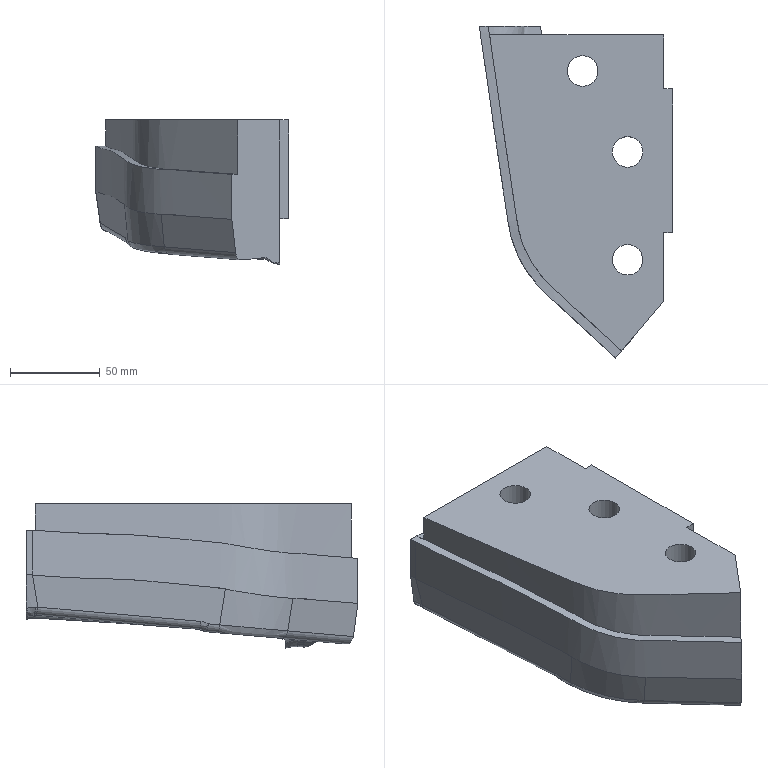Part | NX | features solid 2 | 1 solid | 67 faces | box 107.336 x 184.526 x 80.207 mm | volume 813841 mm3 | spline 28 | plane 19 | cylinder 18 | sphere 2 | commonest cylinder face diameters 10 x9 17 x3 25 x3 14 x1 60 x1 130 x1